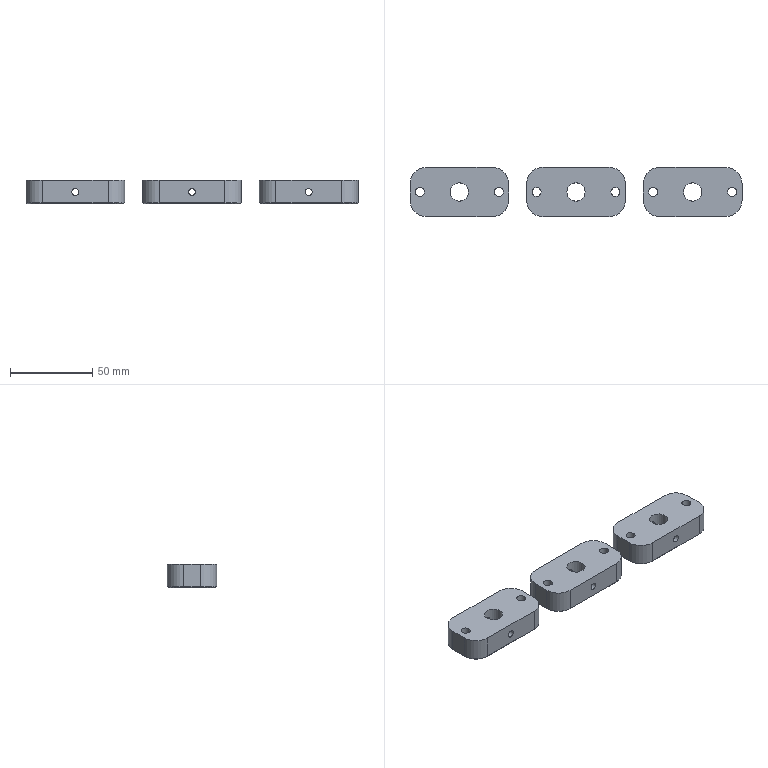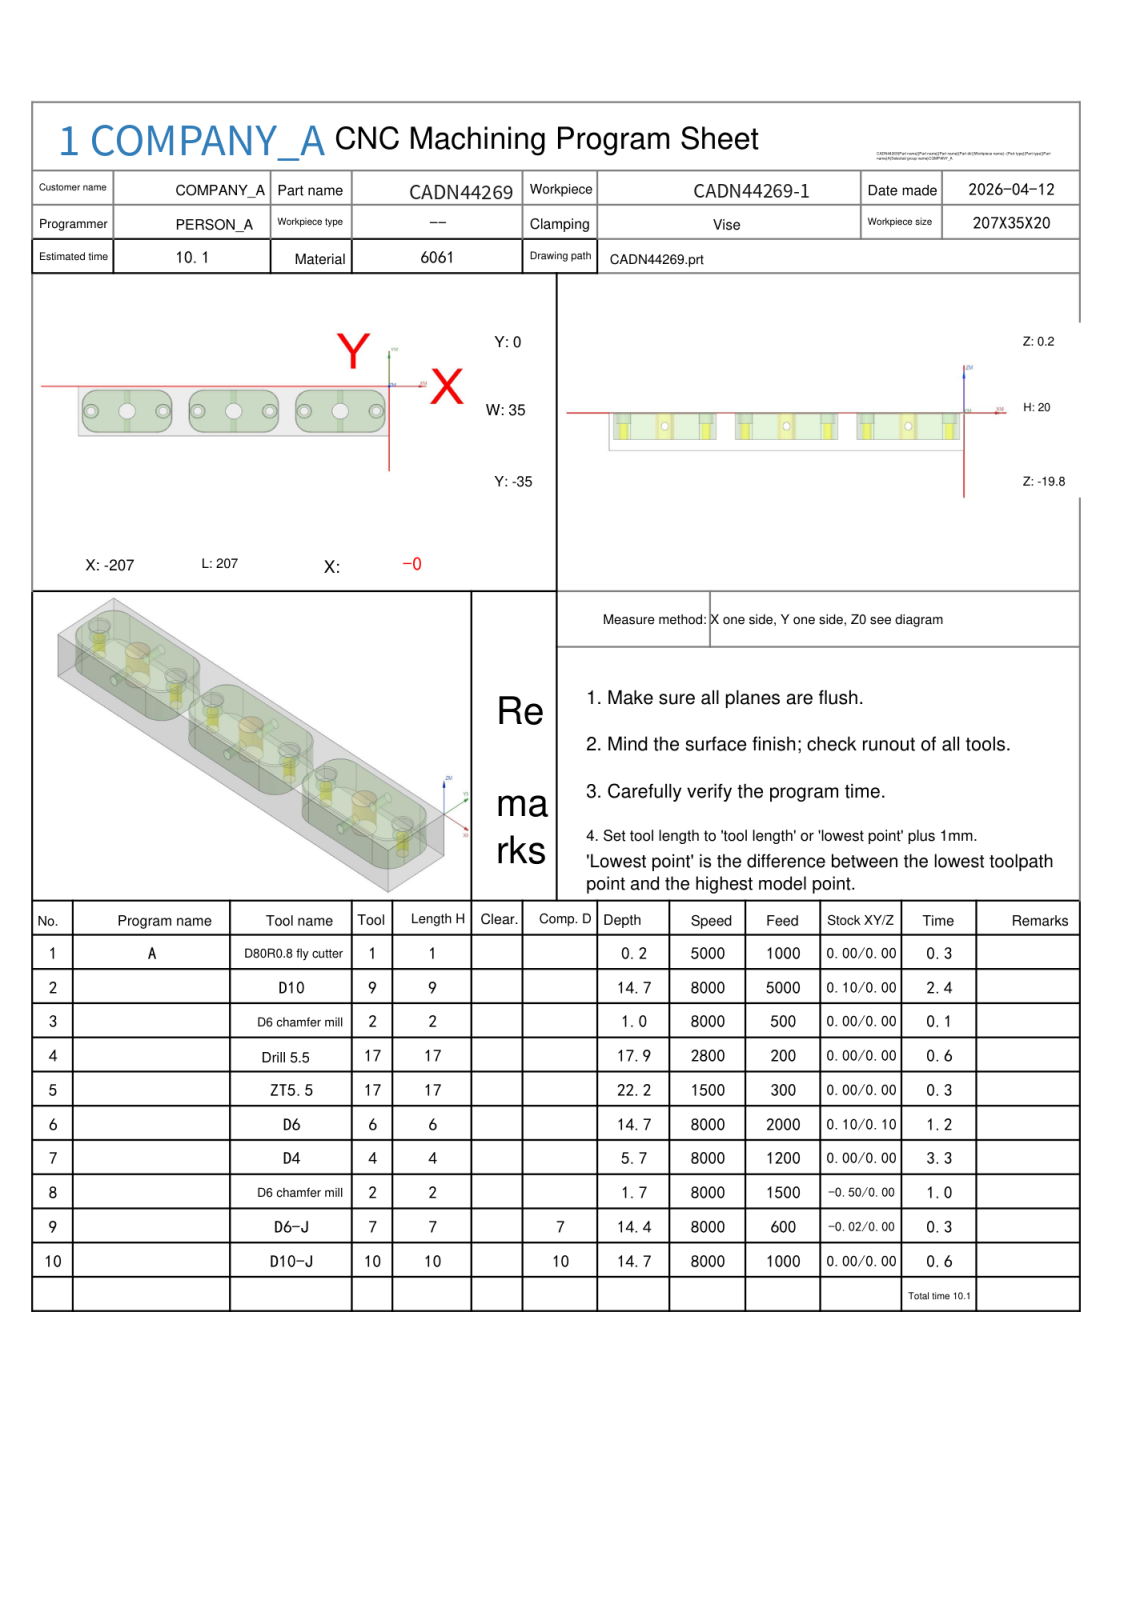NC program | NX | posted by the shop | part box 202 x 30 x 14 mm
Lines 1 to 1289 of 2337, first 1135 of 1287 lines:
%
O0001
(Machine time: 11.90 MIN)
(===Total Tool:8===)
(T1=D80R0.8 fly cutter D=80.  R=0.8  D-  H01 Z=-0.   )
(T9=D10     D=10.  R=0.   D-  H09 Z=-14.5 )
(T2=D6 chamfer mill   D=6.   R=0.   D-  H02 Z=-1.5  )
(T17=drill 5.5  D=5.5  DR_a=118 D-  H17 Z=-22.  )
(T6=D6      D=6.   R=0.   D-  H06 Z=-14.5 )
(T4=D4      D=4.   R=0.   D4  H04 Z=-5.5  )
(T7=D6-J    D=6.   R=0.   D7  H07 Z=-14.2 )
(T10=D10-J  D=10.  R=0.   D10 H10 Z=-14.5 )
G80 G90 G17 G49 G40
G91 G28 Z0
M01
N1 T01 M06
(D80R0.8 fly cutter  D=80. R=0.8 H=01 ce=0.00 di=0.00)
G00 G90 G54 X42.5 Y-17.5 M03 S5000
G43 H01 Z20.
M08
Z2.
G01 Z0.0 F1000.
X37.5
X-244.5
X-249.5
Z2.
G00 Z20.
G91 G28 Z0.0
M05
M09
G91 G28 Z0.0
M01
N2 T09 M06
(D10  D=10. R=0. H=09 ce=0.10 di=0.00)
G00 G90 G54 X-103.5 Y2.6 M03 S8000
G43 H09 Z20.
M08
Z.5
G01 X-83.5 Z.419 F5000.
G02 X-68.4 Y-12.5 Z.323 I0.0 J-15.1
G01 Y-22.5 Z.282
G02 X-83.5 Y-37.6 Z.186 I-15.1 J0.0
G01 X-123.5 Z.024
G02 X-138.6 Y-22.5 Z-.072 I0.0 J15.1
G01 Y-12.5 Z-.112
G02 X-123.5 Y2.6 Z-.208 I15.1 J0.0
G01 X-83.5 Z-.37
G02 X-68.4 Y-12.5 Z-.467 I0.0 J-15.1
G01 Y-22.5 Z-.507
G02 X-83.5 Y-37.6 Z-.603 I-15.1 J0.0
G01 X-123.5 Z-.765
G02 X-138.6 Y-22.5 Z-.861 I0.0 J15.1
G01 Y-12.5 Z-.902
G02 X-123.5 Y2.6 Z-.998 I15.1 J0.0
G01 X-83.5 Z-1.16
G02 X-68.4 Y-12.5 Z-1.256 I0.0 J-15.1
G01 Y-22.5 Z-1.297
G02 X-83.5 Y-37.6 Z-1.393 I-15.1 J0.0
G01 X-123.5 Z-1.555
G02 X-138.6 Y-22.5 Z-1.651 I0.0 J15.1
G01 Y-12.5 Z-1.691
G02 X-123.5 Y2.6 Z-1.787 I15.1 J0.0
G01 X-83.5 Z-1.949
G02 X-68.4 Y-12.5 Z-2.046 I0.0 J-15.1
G01 Y-22.5 Z-2.086
G02 X-83.5 Y-37.6 Z-2.182 I-15.1 J0.0
G01 X-123.5 Z-2.344
G02 X-138.6 Y-22.5 Z-2.44 I0.0 J15.1
G01 Y-12.5 Z-2.481
G02 X-123.5 Y2.6 Z-2.577 I15.1 J0.0
G01 X-83.5 Z-2.739
G02 X-68.4 Y-12.5 Z-2.835 I0.0 J-15.1
G01 Y-22.5 Z-2.876
G02 X-83.5 Y-37.6 Z-2.972 I-15.1 J0.0
G01 X-123.5 Z-3.134
G02 X-138.6 Y-22.5 Z-3.23 I0.0 J15.1
G01 Y-12.5 Z-3.27
G02 X-123.5 Y2.6 Z-3.366 I15.1 J0.0
G01 X-83.5 Z-3.528
G02 X-68.4 Y-12.5 Z-3.624 I0.0 J-15.1
G01 Y-22.5 Z-3.665
G02 X-83.5 Y-37.6 Z-3.761 I-15.1 J0.0
G01 X-123.5 Z-3.923
G02 X-138.6 Y-22.5 Z-4.019 I0.0 J15.1
G01 Y-12.5 Z-4.06
G02 X-123.5 Y2.6 Z-4.156 I15.1 J0.0
G01 X-83.5 Z-4.318
G02 X-68.4 Y-12.5 Z-4.414 I0.0 J-15.1
G01 Y-22.5 Z-4.454
G02 X-83.5 Y-37.6 Z-4.551 I-15.1 J0.0
G01 X-123.5 Z-4.713
G02 X-138.6 Y-22.5 Z-4.809 I0.0 J15.1
G01 Y-12.5 Z-4.849
G02 X-123.5 Y2.6 Z-4.945 I15.1 J0.0
G01 X-83.5 Z-5.107
G02 X-68.4 Y-12.5 Z-5.203 I0.0 J-15.1
G01 Y-22.5 Z-5.244
G02 X-83.5 Y-37.6 Z-5.34 I-15.1 J0.0
G01 X-123.5 Z-5.502
G02 X-138.6 Y-22.5 Z-5.598 I0.0 J15.1
G01 Y-12.5 Z-5.639
G02 X-123.5 Y2.6 Z-5.735 I15.1 J0.0
G01 X-83.5 Z-5.897
G02 X-68.4 Y-12.5 Z-5.993 I0.0 J-15.1
G01 Y-22.5 Z-6.033
G02 X-83.5 Y-37.6 Z-6.13 I-15.1 J0.0
G01 X-123.5 Z-6.292
G02 X-138.6 Y-22.5 Z-6.388 I0.0 J15.1
G01 Y-12.5 Z-6.428
G02 X-123.5 Y2.6 Z-6.524 I15.1 J0.0
G01 X-83.5 Z-6.686
G02 X-68.4 Y-12.5 Z-6.782 I0.0 J-15.1
G01 Y-22.5 Z-6.823
G02 X-83.5 Y-37.6 Z-6.919 I-15.1 J0.0
G01 X-123.5 Z-7.081
G02 X-138.6 Y-22.5 Z-7.177 I0.0 J15.1
G01 Y-12.5 Z-7.218
G02 X-123.5 Y2.6 Z-7.314 I15.1 J0.0
G01 X-83.5 Z-7.476
G02 X-68.4 Y-12.5 Z-7.572 I0.0 J-15.1
G01 Y-22.5 Z-7.612
G02 X-83.5 Y-37.6 Z-7.708 I-15.1 J0.0
G01 X-123.5 Z-7.87
G02 X-138.6 Y-22.5 Z-7.967 I0.0 J15.1
G01 Y-12.5 Z-8.007
G02 X-123.5 Y2.6 Z-8.103 I15.1 J0.0
G01 X-83.5 Z-8.265
G02 X-68.4 Y-12.5 Z-8.361 I0.0 J-15.1
G01 Y-22.5 Z-8.402
G02 X-83.5 Y-37.6 Z-8.498 I-15.1 J0.0
G01 X-123.5 Z-8.66
G02 X-138.6 Y-22.5 Z-8.756 I0.0 J15.1
G01 Y-12.5 Z-8.797
G02 X-123.5 Y2.6 Z-8.893 I15.1 J0.0
G01 X-83.5 Z-9.055
G02 X-68.4 Y-12.5 Z-9.151 I0.0 J-15.1
G01 Y-22.5 Z-9.191
G02 X-83.5 Y-37.6 Z-9.287 I-15.1 J0.0
G01 X-123.5 Z-9.449
G02 X-138.6 Y-22.5 Z-9.546 I0.0 J15.1
G01 Y-12.5 Z-9.586
G02 X-123.5 Y2.6 Z-9.682 I15.1 J0.0
G01 X-83.5 Z-9.844
G02 X-68.4 Y-12.5 Z-9.94 I0.0 J-15.1
G01 Y-22.5 Z-9.981
G02 X-83.5 Y-37.6 Z-10.077 I-15.1 J0.0
G01 X-123.5 Z-10.239
G02 X-138.6 Y-22.5 Z-10.335 I0.0 J15.1
G01 Y-12.5 Z-10.376
G02 X-123.5 Y2.6 Z-10.472 I15.1 J0.0
G01 X-83.5 Z-10.634
G02 X-68.4 Y-12.5 Z-10.73 I0.0 J-15.1
G01 Y-22.5 Z-10.77
G02 X-83.5 Y-37.6 Z-10.866 I-15.1 J0.0
G01 X-123.5 Z-11.028
G02 X-138.6 Y-22.5 Z-11.124 I0.0 J15.1
G01 Y-12.5 Z-11.165
G02 X-123.5 Y2.6 Z-11.261 I15.1 J0.0
G01 X-83.5 Z-11.423
G02 X-68.4 Y-12.5 Z-11.519 I0.0 J-15.1
G01 Y-22.5 Z-11.56
G02 X-83.5 Y-37.6 Z-11.656 I-15.1 J0.0
G01 X-123.5 Z-11.818
G02 X-138.6 Y-22.5 Z-11.914 I0.0 J15.1
G01 Y-12.5 Z-11.954
G02 X-123.5 Y2.6 Z-12.051 I15.1 J0.0
G01 X-83.5 Z-12.213
G02 X-68.4 Y-12.5 Z-12.309 I0.0 J-15.1
G01 Y-22.5 Z-12.349
G02 X-83.5 Y-37.6 Z-12.445 I-15.1 J0.0
G01 X-123.5 Z-12.607
G02 X-138.6 Y-22.5 Z-12.703 I0.0 J15.1
G01 Y-12.5 Z-12.744
G02 X-123.5 Y2.6 Z-12.84 I15.1 J0.0
G01 X-83.5 Z-13.002
G02 X-68.4 Y-12.5 Z-13.098 I0.0 J-15.1
G01 Y-22.5 Z-13.139
G02 X-83.5 Y-37.6 Z-13.235 I-15.1 J0.0
G01 X-123.5 Z-13.397
G02 X-138.6 Y-22.5 Z-13.493 I0.0 J15.1
G01 Y-12.5 Z-13.533
G02 X-123.5 Y2.6 Z-13.63 I15.1 J0.0
G01 X-83.5 Z-13.792
G02 X-68.4 Y-12.5 Z-13.888 I0.0 J-15.1
G01 Y-22.5 Z-13.928
G02 X-83.5 Y-37.6 Z-14.024 I-15.1 J0.0
G01 X-123.5 Z-14.186
G02 X-138.6 Y-22.5 Z-14.282 I0.0 J15.1
G01 Y-12.5 Z-14.323
G02 X-123.5 Y2.6 Z-14.419 I15.1 J0.0
G01 X-103.5 Z-14.5
X-83.5
G02 X-68.4 Y-12.5 I0.0 J-15.1
G01 Y-22.5
G02 X-83.5 Y-37.6 I-15.1 J0.0
G01 X-123.5
G02 X-138.6 Y-22.5 I0.0 J15.1
G01 Y-12.5
G02 X-123.5 Y2.6 I15.1 J0.0
G01 X-103.5
X-103.
Z-13.5
G00 Z20.
X-32.5
Z.5
G01 X-12.5 Z.419
G02 X2.6 Y-12.5 Z.323 I0.0 J-15.1
G01 Y-22.5 Z.282
G02 X-12.5 Y-37.6 Z.186 I-15.1 J0.0
G01 X-52.5 Z.024
G02 X-67.6 Y-22.5 Z-.072 I0.0 J15.1
G01 Y-12.5 Z-.112
G02 X-52.5 Y2.6 Z-.208 I15.1 J0.0
G01 X-12.5 Z-.37
G02 X2.6 Y-12.5 Z-.467 I0.0 J-15.1
G01 Y-22.5 Z-.507
G02 X-12.5 Y-37.6 Z-.603 I-15.1 J0.0
G01 X-52.5 Z-.765
G02 X-67.6 Y-22.5 Z-.861 I0.0 J15.1
G01 Y-12.5 Z-.902
G02 X-52.5 Y2.6 Z-.998 I15.1 J0.0
G01 X-12.5 Z-1.16
G02 X2.6 Y-12.5 Z-1.256 I0.0 J-15.1
G01 Y-22.5 Z-1.297
G02 X-12.5 Y-37.6 Z-1.393 I-15.1 J0.0
G01 X-52.5 Z-1.555
G02 X-67.6 Y-22.5 Z-1.651 I0.0 J15.1
G01 Y-12.5 Z-1.691
G02 X-52.5 Y2.6 Z-1.787 I15.1 J0.0
G01 X-12.5 Z-1.949
G02 X2.6 Y-12.5 Z-2.046 I0.0 J-15.1
G01 Y-22.5 Z-2.086
G02 X-12.5 Y-37.6 Z-2.182 I-15.1 J0.0
G01 X-52.5 Z-2.344
G02 X-67.6 Y-22.5 Z-2.44 I0.0 J15.1
G01 Y-12.5 Z-2.481
G02 X-52.5 Y2.6 Z-2.577 I15.1 J0.0
G01 X-12.5 Z-2.739
G02 X2.6 Y-12.5 Z-2.835 I0.0 J-15.1
G01 Y-22.5 Z-2.876
G02 X-12.5 Y-37.6 Z-2.972 I-15.1 J0.0
G01 X-52.5 Z-3.134
G02 X-67.6 Y-22.5 Z-3.23 I0.0 J15.1
G01 Y-12.5 Z-3.27
G02 X-52.5 Y2.6 Z-3.366 I15.1 J0.0
G01 X-12.5 Z-3.528
G02 X2.6 Y-12.5 Z-3.624 I0.0 J-15.1
G01 Y-22.5 Z-3.665
G02 X-12.5 Y-37.6 Z-3.761 I-15.1 J0.0
G01 X-52.5 Z-3.923
G02 X-67.6 Y-22.5 Z-4.019 I0.0 J15.1
G01 Y-12.5 Z-4.06
G02 X-52.5 Y2.6 Z-4.156 I15.1 J0.0
G01 X-12.5 Z-4.318
G02 X2.6 Y-12.5 Z-4.414 I0.0 J-15.1
G01 Y-22.5 Z-4.454
G02 X-12.5 Y-37.6 Z-4.551 I-15.1 J0.0
G01 X-52.5 Z-4.713
G02 X-67.6 Y-22.5 Z-4.809 I0.0 J15.1
G01 Y-12.5 Z-4.849
G02 X-52.5 Y2.6 Z-4.945 I15.1 J0.0
G01 X-12.5 Z-5.107
G02 X2.6 Y-12.5 Z-5.203 I0.0 J-15.1
G01 Y-22.5 Z-5.244
G02 X-12.5 Y-37.6 Z-5.34 I-15.1 J0.0
G01 X-52.5 Z-5.502
G02 X-67.6 Y-22.5 Z-5.598 I0.0 J15.1
G01 Y-12.5 Z-5.639
G02 X-52.5 Y2.6 Z-5.735 I15.1 J0.0
G01 X-12.5 Z-5.897
G02 X2.6 Y-12.5 Z-5.993 I0.0 J-15.1
G01 Y-22.5 Z-6.033
G02 X-12.5 Y-37.6 Z-6.13 I-15.1 J0.0
G01 X-52.5 Z-6.292
G02 X-67.6 Y-22.5 Z-6.388 I0.0 J15.1
G01 Y-12.5 Z-6.428
G02 X-52.5 Y2.6 Z-6.524 I15.1 J0.0
G01 X-12.5 Z-6.686
G02 X2.6 Y-12.5 Z-6.782 I0.0 J-15.1
G01 Y-22.5 Z-6.823
G02 X-12.5 Y-37.6 Z-6.919 I-15.1 J0.0
G01 X-52.5 Z-7.081
G02 X-67.6 Y-22.5 Z-7.177 I0.0 J15.1
G01 Y-12.5 Z-7.218
G02 X-52.5 Y2.6 Z-7.314 I15.1 J0.0
G01 X-12.5 Z-7.476
G02 X2.6 Y-12.5 Z-7.572 I0.0 J-15.1
G01 Y-22.5 Z-7.612
G02 X-12.5 Y-37.6 Z-7.708 I-15.1 J0.0
G01 X-52.5 Z-7.87
G02 X-67.6 Y-22.5 Z-7.967 I0.0 J15.1
G01 Y-12.5 Z-8.007
G02 X-52.5 Y2.6 Z-8.103 I15.1 J0.0
G01 X-12.5 Z-8.265
G02 X2.6 Y-12.5 Z-8.361 I0.0 J-15.1
G01 Y-22.5 Z-8.402
G02 X-12.5 Y-37.6 Z-8.498 I-15.1 J0.0
G01 X-52.5 Z-8.66
G02 X-67.6 Y-22.5 Z-8.756 I0.0 J15.1
G01 Y-12.5 Z-8.797
G02 X-52.5 Y2.6 Z-8.893 I15.1 J0.0
G01 X-12.5 Z-9.055
G02 X2.6 Y-12.5 Z-9.151 I0.0 J-15.1
G01 Y-22.5 Z-9.191
G02 X-12.5 Y-37.6 Z-9.287 I-15.1 J0.0
G01 X-52.5 Z-9.449
G02 X-67.6 Y-22.5 Z-9.546 I0.0 J15.1
G01 Y-12.5 Z-9.586
G02 X-52.5 Y2.6 Z-9.682 I15.1 J0.0
G01 X-12.5 Z-9.844
G02 X2.6 Y-12.5 Z-9.94 I0.0 J-15.1
G01 Y-22.5 Z-9.981
G02 X-12.5 Y-37.6 Z-10.077 I-15.1 J0.0
G01 X-52.5 Z-10.239
G02 X-67.6 Y-22.5 Z-10.335 I0.0 J15.1
G01 Y-12.5 Z-10.376
G02 X-52.5 Y2.6 Z-10.472 I15.1 J0.0
G01 X-12.5 Z-10.634
G02 X2.6 Y-12.5 Z-10.73 I0.0 J-15.1
G01 Y-22.5 Z-10.77
G02 X-12.5 Y-37.6 Z-10.866 I-15.1 J0.0
G01 X-52.5 Z-11.028
G02 X-67.6 Y-22.5 Z-11.124 I0.0 J15.1
G01 Y-12.5 Z-11.165
G02 X-52.5 Y2.6 Z-11.261 I15.1 J0.0
G01 X-12.5 Z-11.423
G02 X2.6 Y-12.5 Z-11.519 I0.0 J-15.1
G01 Y-22.5 Z-11.56
G02 X-12.5 Y-37.6 Z-11.656 I-15.1 J0.0
G01 X-52.5 Z-11.818
G02 X-67.6 Y-22.5 Z-11.914 I0.0 J15.1
G01 Y-12.5 Z-11.954
G02 X-52.5 Y2.6 Z-12.051 I15.1 J0.0
G01 X-12.5 Z-12.213
G02 X2.6 Y-12.5 Z-12.309 I0.0 J-15.1
G01 Y-22.5 Z-12.349
G02 X-12.5 Y-37.6 Z-12.445 I-15.1 J0.0
G01 X-52.5 Z-12.607
G02 X-67.6 Y-22.5 Z-12.703 I0.0 J15.1
G01 Y-12.5 Z-12.744
G02 X-52.5 Y2.6 Z-12.84 I15.1 J0.0
G01 X-12.5 Z-13.002
G02 X2.6 Y-12.5 Z-13.098 I0.0 J-15.1
G01 Y-22.5 Z-13.139
G02 X-12.5 Y-37.6 Z-13.235 I-15.1 J0.0
G01 X-52.5 Z-13.397
G02 X-67.6 Y-22.5 Z-13.493 I0.0 J15.1
G01 Y-12.5 Z-13.533
G02 X-52.5 Y2.6 Z-13.63 I15.1 J0.0
G01 X-12.5 Z-13.792
G02 X2.6 Y-12.5 Z-13.888 I0.0 J-15.1
G01 Y-22.5 Z-13.928
G02 X-12.5 Y-37.6 Z-14.024 I-15.1 J0.0
G01 X-52.5 Z-14.186
G02 X-67.6 Y-22.5 Z-14.282 I0.0 J15.1
G01 Y-12.5 Z-14.323
G02 X-52.5 Y2.6 Z-14.419 I15.1 J0.0
G01 X-32.5 Z-14.5
X-12.5
G02 X2.6 Y-12.5 I0.0 J-15.1
G01 Y-22.5
G02 X-12.5 Y-37.6 I-15.1 J0.0
G01 X-52.5
G02 X-67.6 Y-22.5 I0.0 J15.1
G01 Y-12.5
G02 X-52.5 Y2.6 I15.1 J0.0
G01 X-32.5
X-32.
Z-13.5
G00 Z20.
X-174.5
Z.5
G01 X-154.5 Z.419
G02 X-139.4 Y-12.5 Z.323 I0.0 J-15.1
G01 Y-22.5 Z.282
G02 X-154.5 Y-37.6 Z.186 I-15.1 J0.0
G01 X-194.5 Z.024
G02 X-209.6 Y-22.5 Z-.072 I0.0 J15.1
G01 Y-12.5 Z-.112
G02 X-194.5 Y2.6 Z-.208 I15.1 J0.0
G01 X-154.5 Z-.37
G02 X-139.4 Y-12.5 Z-.467 I0.0 J-15.1
G01 Y-22.5 Z-.507
G02 X-154.5 Y-37.6 Z-.603 I-15.1 J0.0
G01 X-194.5 Z-.765
G02 X-209.6 Y-22.5 Z-.861 I0.0 J15.1
G01 Y-12.5 Z-.902
G02 X-194.5 Y2.6 Z-.998 I15.1 J0.0
G01 X-154.5 Z-1.16
G02 X-139.4 Y-12.5 Z-1.256 I0.0 J-15.1
G01 Y-22.5 Z-1.297
G02 X-154.5 Y-37.6 Z-1.393 I-15.1 J0.0
G01 X-194.5 Z-1.555
G02 X-209.6 Y-22.5 Z-1.651 I0.0 J15.1
G01 Y-12.5 Z-1.691
G02 X-194.5 Y2.6 Z-1.787 I15.1 J0.0
G01 X-154.5 Z-1.949
G02 X-139.4 Y-12.5 Z-2.046 I0.0 J-15.1
G01 Y-22.5 Z-2.086
G02 X-154.5 Y-37.6 Z-2.182 I-15.1 J0.0
G01 X-194.5 Z-2.344
G02 X-209.6 Y-22.5 Z-2.44 I0.0 J15.1
G01 Y-12.5 Z-2.481
G02 X-194.5 Y2.6 Z-2.577 I15.1 J0.0
G01 X-154.5 Z-2.739
G02 X-139.4 Y-12.5 Z-2.835 I0.0 J-15.1
G01 Y-22.5 Z-2.876
G02 X-154.5 Y-37.6 Z-2.972 I-15.1 J0.0
G01 X-194.5 Z-3.134
G02 X-209.6 Y-22.5 Z-3.23 I0.0 J15.1
G01 Y-12.5 Z-3.27
G02 X-194.5 Y2.6 Z-3.366 I15.1 J0.0
G01 X-154.5 Z-3.528
G02 X-139.4 Y-12.5 Z-3.624 I0.0 J-15.1
G01 Y-22.5 Z-3.665
G02 X-154.5 Y-37.6 Z-3.761 I-15.1 J0.0
G01 X-194.5 Z-3.923
G02 X-209.6 Y-22.5 Z-4.019 I0.0 J15.1
G01 Y-12.5 Z-4.06
G02 X-194.5 Y2.6 Z-4.156 I15.1 J0.0
G01 X-154.5 Z-4.318
G02 X-139.4 Y-12.5 Z-4.414 I0.0 J-15.1
G01 Y-22.5 Z-4.454
G02 X-154.5 Y-37.6 Z-4.551 I-15.1 J0.0
G01 X-194.5 Z-4.713
G02 X-209.6 Y-22.5 Z-4.809 I0.0 J15.1
G01 Y-12.5 Z-4.849
G02 X-194.5 Y2.6 Z-4.945 I15.1 J0.0
G01 X-154.5 Z-5.107
G02 X-139.4 Y-12.5 Z-5.203 I0.0 J-15.1
G01 Y-22.5 Z-5.244
G02 X-154.5 Y-37.6 Z-5.34 I-15.1 J0.0
G01 X-194.5 Z-5.502
G02 X-209.6 Y-22.5 Z-5.598 I0.0 J15.1
G01 Y-12.5 Z-5.639
G02 X-194.5 Y2.6 Z-5.735 I15.1 J0.0
G01 X-154.5 Z-5.897
G02 X-139.4 Y-12.5 Z-5.993 I0.0 J-15.1
G01 Y-22.5 Z-6.033
G02 X-154.5 Y-37.6 Z-6.13 I-15.1 J0.0
G01 X-194.5 Z-6.292
G02 X-209.6 Y-22.5 Z-6.388 I0.0 J15.1
G01 Y-12.5 Z-6.428
G02 X-194.5 Y2.6 Z-6.524 I15.1 J0.0
G01 X-154.5 Z-6.686
G02 X-139.4 Y-12.5 Z-6.782 I0.0 J-15.1
G01 Y-22.5 Z-6.823
G02 X-154.5 Y-37.6 Z-6.919 I-15.1 J0.0
G01 X-194.5 Z-7.081
G02 X-209.6 Y-22.5 Z-7.177 I0.0 J15.1
G01 Y-12.5 Z-7.218
G02 X-194.5 Y2.6 Z-7.314 I15.1 J0.0
G01 X-154.5 Z-7.476
G02 X-139.4 Y-12.5 Z-7.572 I0.0 J-15.1
G01 Y-22.5 Z-7.612
G02 X-154.5 Y-37.6 Z-7.708 I-15.1 J0.0
G01 X-194.5 Z-7.87
G02 X-209.6 Y-22.5 Z-7.967 I0.0 J15.1
G01 Y-12.5 Z-8.007
G02 X-194.5 Y2.6 Z-8.103 I15.1 J0.0
G01 X-154.5 Z-8.265
G02 X-139.4 Y-12.5 Z-8.361 I0.0 J-15.1
G01 Y-22.5 Z-8.402
G02 X-154.5 Y-37.6 Z-8.498 I-15.1 J0.0
G01 X-194.5 Z-8.66
G02 X-209.6 Y-22.5 Z-8.756 I0.0 J15.1
G01 Y-12.5 Z-8.797
G02 X-194.5 Y2.6 Z-8.893 I15.1 J0.0
G01 X-154.5 Z-9.055
G02 X-139.4 Y-12.5 Z-9.151 I0.0 J-15.1
G01 Y-22.5 Z-9.191
G02 X-154.5 Y-37.6 Z-9.287 I-15.1 J0.0
G01 X-194.5 Z-9.449
G02 X-209.6 Y-22.5 Z-9.546 I0.0 J15.1
G01 Y-12.5 Z-9.586
G02 X-194.5 Y2.6 Z-9.682 I15.1 J0.0
G01 X-154.5 Z-9.844
G02 X-139.4 Y-12.5 Z-9.94 I0.0 J-15.1
G01 Y-22.5 Z-9.981
G02 X-154.5 Y-37.6 Z-10.077 I-15.1 J0.0
G01 X-194.5 Z-10.239
G02 X-209.6 Y-22.5 Z-10.335 I0.0 J15.1
G01 Y-12.5 Z-10.376
G02 X-194.5 Y2.6 Z-10.472 I15.1 J0.0
G01 X-154.5 Z-10.634
G02 X-139.4 Y-12.5 Z-10.73 I0.0 J-15.1
G01 Y-22.5 Z-10.77
G02 X-154.5 Y-37.6 Z-10.866 I-15.1 J0.0
G01 X-194.5 Z-11.028
G02 X-209.6 Y-22.5 Z-11.124 I0.0 J15.1
G01 Y-12.5 Z-11.165
G02 X-194.5 Y2.6 Z-11.261 I15.1 J0.0
G01 X-154.5 Z-11.423
G02 X-139.4 Y-12.5 Z-11.519 I0.0 J-15.1
G01 Y-22.5 Z-11.56
G02 X-154.5 Y-37.6 Z-11.656 I-15.1 J0.0
G01 X-194.5 Z-11.818
G02 X-209.6 Y-22.5 Z-11.914 I0.0 J15.1
G01 Y-12.5 Z-11.954
G02 X-194.5 Y2.6 Z-12.051 I15.1 J0.0
G01 X-154.5 Z-12.213
G02 X-139.4 Y-12.5 Z-12.309 I0.0 J-15.1
G01 Y-22.5 Z-12.349
G02 X-154.5 Y-37.6 Z-12.445 I-15.1 J0.0
G01 X-194.5 Z-12.607
G02 X-209.6 Y-22.5 Z-12.703 I0.0 J15.1
G01 Y-12.5 Z-12.744
G02 X-194.5 Y2.6 Z-12.84 I15.1 J0.0
G01 X-154.5 Z-13.002
G02 X-139.4 Y-12.5 Z-13.098 I0.0 J-15.1
G01 Y-22.5 Z-13.139
G02 X-154.5 Y-37.6 Z-13.235 I-15.1 J0.0
G01 X-194.5 Z-13.397
G02 X-209.6 Y-22.5 Z-13.493 I0.0 J15.1
G01 Y-12.5 Z-13.533
G02 X-194.5 Y2.6 Z-13.63 I15.1 J0.0
G01 X-154.5 Z-13.792
G02 X-139.4 Y-12.5 Z-13.888 I0.0 J-15.1
G01 Y-22.5 Z-13.928
G02 X-154.5 Y-37.6 Z-14.024 I-15.1 J0.0
G01 X-194.5 Z-14.186
G02 X-209.6 Y-22.5 Z-14.282 I0.0 J15.1
G01 Y-12.5 Z-14.323
G02 X-194.5 Y2.6 Z-14.419 I15.1 J0.0
G01 X-174.5 Z-14.5
X-154.5
G02 X-139.4 Y-12.5 I0.0 J-15.1
G01 Y-22.5
G02 X-154.5 Y-37.6 I-15.1 J0.0
G01 X-194.5
G02 X-209.6 Y-22.5 I0.0 J15.1
G01 Y-12.5
G02 X-194.5 Y2.6 I15.1 J0.0
G01 X-174.5
X-174.
Z-13.5
G00 Z20.
G91 G28 Z0.0
M05
M09
G91 G28 Z0.0
M01
N3 T02 M06
(D6 chamfer mill  D=6. R=0. H=02 ce=0.00 di=0.00)
G00 G90 G54 X-174.5 Y-17.5 M03 S8000
G43 H02 Z20.
M08
G98 G82 X-174.5 Y-17.5 Z-.8 R1. F500.
X-103.5
X-32.5
G80
G00 Z20.
G00 G90 X-198.5 Y-17.5 M03 S8000
Z20.
G98 G81 X-198.5 Y-17.5 Z-.8 R1. F500.
X-150.5
X-127.5
X-79.5
X-56.5
X-8.5
G80
G00 Z20.
G91 G28 Z0.0
M05
M09
G91 G28 Z0.0
M01
N4 T17 M06
(drill 5.5 D=5.5 DR_a=118 H=17)
G00 G90 G54 X-198.5 Y-17.5 M03 S2800
G43 H17 Z20.
M08
G98 G83 X-198.5 Y-17.5 Z-17.652 R1. F200. Q2.
X-150.5
X-127.5
X-79.5
X-56.5
X-8.5
G80
G00 Z20.
G91 G28 Z0.0
M05
M09
G91 G28 Z0.0
M01
N5 T17 M06
(ZT5.5 D=5.5 DR_a=118 H=17)
G00 G90 G54 X-174.5 Y-17.5 M03 S1500
G43 H17 Z20.
M08
G98 G83 X-174.5 Y-17.5 Z-22. R1. F300. Q3.
X-103.5
X-32.5
G80
G00 Z20.
G91 G28 Z0.0
M05
M09
G91 G28 Z0.0
M01
N6 T06 M06
(D6  D=6. R=0. H=06 ce=0.10 di=0.10)
G00 G90 G54 X-34.93 Y-17.611 M03 S8000
G43 H06 Z20.
M08
Z1.
G01 Y-17.883 Z.986 F2000.
X-34.563 Y-18.839 Z.932
X-33.839 Y-19.563 Z.878
X-32.883 Y-19.93 Z.825
X-32.117 Z.785
X-31.161 Y-19.563 Z.731
X-30.437 Y-18.839 Z.677
X-30.07 Y-17.883 Z.624
Y-17.117 Z.583
X-30.437 Y-16.161 Z.53
X-31.161 Y-15.437 Z.476
X-32.117 Y-15.07 Z.422
X-32.883 Z.382
X-33.839 Y-15.437 Z.329
X-34.563 Y-16.161 Z.275
X-34.93 Y-17.117 Z.221
Y-17.883 Z.181
X-34.563 Y-18.839 Z.127
X-33.839 Y-19.563 Z.074
X-32.883 Y-19.93 Z.02
X-32.5 Z0.0
G03 X-30.07 Y-17.5 Z-.074 I0.0 J2.43
X-32.5 Y-15.07 Z-.148 I-2.43 J0.0
X-34.93 Y-17.5 Z-.222 I0.0 J-2.43
X-32.5 Y-19.93 Z-.296 I2.43 J0.0
X-30.07 Y-17.5 Z-.37 I0.0 J2.43
X-32.5 Y-15.07 Z-.444 I-2.43 J0.0
X-34.93 Y-17.5 Z-.518 I0.0 J-2.43
X-32.5 Y-19.93 Z-.592 I2.43 J0.0
X-30.07 Y-17.5 Z-.666 I0.0 J2.43
X-32.5 Y-15.07 Z-.74 I-2.43 J0.0
X-34.93 Y-17.5 Z-.814 I0.0 J-2.43
X-32.5 Y-19.93 Z-.888 I2.43 J0.0
X-30.07 Y-17.5 Z-.962 I0.0 J2.43
X-32.5 Y-15.07 Z-1.036 I-2.43 J0.0
X-34.93 Y-17.5 Z-1.11 I0.0 J-2.43
X-32.5 Y-19.93 Z-1.184 I2.43 J0.0
X-30.07 Y-17.5 Z-1.258 I0.0 J2.43
X-32.5 Y-15.07 Z-1.332 I-2.43 J0.0
X-34.93 Y-17.5 Z-1.406 I0.0 J-2.43
X-32.5 Y-19.93 Z-1.48 I2.43 J0.0
X-30.07 Y-17.5 Z-1.554 I0.0 J2.43
X-32.5 Y-15.07 Z-1.628 I-2.43 J0.0
X-34.93 Y-17.5 Z-1.702 I0.0 J-2.43
X-32.5 Y-19.93 Z-1.776 I2.43 J0.0
X-30.07 Y-17.5 Z-1.849 I0.0 J2.43
X-32.5 Y-15.07 Z-1.923 I-2.43 J0.0
X-34.93 Y-17.5 Z-1.997 I0.0 J-2.43
X-32.5 Y-19.93 Z-2.071 I2.43 J0.0
X-30.07 Y-17.5 Z-2.145 I0.0 J2.43
X-32.5 Y-15.07 Z-2.219 I-2.43 J0.0
X-34.93 Y-17.5 Z-2.293 I0.0 J-2.43
X-32.5 Y-19.93 Z-2.367 I2.43 J0.0
X-30.07 Y-17.5 Z-2.441 I0.0 J2.43
X-32.5 Y-15.07 Z-2.515 I-2.43 J0.0
X-34.93 Y-17.5 Z-2.589 I0.0 J-2.43
X-32.5 Y-19.93 Z-2.663 I2.43 J0.0
X-30.07 Y-17.5 Z-2.737 I0.0 J2.43
X-32.5 Y-15.07 Z-2.811 I-2.43 J0.0
X-34.93 Y-17.5 Z-2.885 I0.0 J-2.43
X-32.5 Y-19.93 Z-2.959 I2.43 J0.0
X-30.07 Y-17.5 Z-3.033 I0.0 J2.43
X-32.5 Y-15.07 Z-3.107 I-2.43 J0.0
X-34.93 Y-17.5 Z-3.181 I0.0 J-2.43
X-32.5 Y-19.93 Z-3.255 I2.43 J0.0
X-30.07 Y-17.5 Z-3.329 I0.0 J2.43
X-32.5 Y-15.07 Z-3.403 I-2.43 J0.0
X-34.93 Y-17.5 Z-3.477 I0.0 J-2.43
X-32.5 Y-19.93 Z-3.551 I2.43 J0.0
X-30.07 Y-17.5 Z-3.625 I0.0 J2.43
X-32.5 Y-15.07 Z-3.699 I-2.43 J0.0
X-34.93 Y-17.5 Z-3.773 I0.0 J-2.43
X-32.5 Y-19.93 Z-3.847 I2.43 J0.0
X-30.07 Y-17.5 Z-3.921 I0.0 J2.43
X-32.5 Y-15.07 Z-3.995 I-2.43 J0.0
X-34.93 Y-17.5 Z-4.069 I0.0 J-2.43
X-32.5 Y-19.93 Z-4.143 I2.43 J0.0
X-30.07 Y-17.5 Z-4.217 I0.0 J2.43
X-32.5 Y-15.07 Z-4.291 I-2.43 J0.0
X-34.93 Y-17.5 Z-4.365 I0.0 J-2.43
X-32.5 Y-19.93 Z-4.439 I2.43 J0.0
X-30.07 Y-17.5 Z-4.513 I0.0 J2.43
X-32.5 Y-15.07 Z-4.587 I-2.43 J0.0
X-34.93 Y-17.5 Z-4.661 I0.0 J-2.43
X-32.5 Y-19.93 Z-4.735 I2.43 J0.0
X-30.07 Y-17.5 Z-4.809 I0.0 J2.43
X-32.5 Y-15.07 Z-4.883 I-2.43 J0.0
X-34.93 Y-17.5 Z-4.957 I0.0 J-2.43
X-32.5 Y-19.93 Z-5.031 I2.43 J0.0
X-30.07 Y-17.5 Z-5.105 I0.0 J2.43
X-32.5 Y-15.07 Z-5.179 I-2.43 J0.0
X-34.93 Y-17.5 Z-5.253 I0.0 J-2.43
X-32.5 Y-19.93 Z-5.327 I2.43 J0.0
X-30.07 Y-17.5 Z-5.401 I0.0 J2.43
X-32.5 Y-15.07 Z-5.474 I-2.43 J0.0
X-34.93 Y-17.5 Z-5.548 I0.0 J-2.43
X-32.5 Y-19.93 Z-5.622 I2.43 J0.0
X-30.07 Y-17.5 Z-5.696 I0.0 J2.43
X-32.5 Y-15.07 Z-5.77 I-2.43 J0.0
X-34.93 Y-17.5 Z-5.844 I0.0 J-2.43
X-32.5 Y-19.93 Z-5.918 I2.43 J0.0
X-30.07 Y-17.5 Z-5.992 I0.0 J2.43
X-32.5 Y-15.07 Z-6.066 I-2.43 J0.0
X-34.93 Y-17.5 Z-6.14 I0.0 J-2.43
X-32.5 Y-19.93 Z-6.214 I2.43 J0.0
X-30.07 Y-17.5 Z-6.288 I0.0 J2.43
X-32.5 Y-15.07 Z-6.362 I-2.43 J0.0
X-34.93 Y-17.5 Z-6.436 I0.0 J-2.43
X-32.5 Y-19.93 Z-6.51 I2.43 J0.0
X-30.07 Y-17.5 Z-6.584 I0.0 J2.43
X-32.5 Y-15.07 Z-6.658 I-2.43 J0.0
X-34.93 Y-17.5 Z-6.732 I0.0 J-2.43
X-32.5 Y-19.93 Z-6.806 I2.43 J0.0
X-30.07 Y-17.5 Z-6.88 I0.0 J2.43
X-32.5 Y-15.07 Z-6.954 I-2.43 J0.0
X-34.93 Y-17.5 Z-7.028 I0.0 J-2.43
X-32.5 Y-19.93 Z-7.102 I2.43 J0.0
X-30.07 Y-17.5 Z-7.176 I0.0 J2.43
X-32.5 Y-15.07 Z-7.25 I-2.43 J0.0
X-34.93 Y-17.5 Z-7.324 I0.0 J-2.43
X-32.5 Y-19.93 Z-7.398 I2.43 J0.0
X-30.07 Y-17.5 Z-7.472 I0.0 J2.43
X-32.5 Y-15.07 Z-7.546 I-2.43 J0.0
X-34.93 Y-17.5 Z-7.62 I0.0 J-2.43
X-32.5 Y-19.93 Z-7.694 I2.43 J0.0
X-30.07 Y-17.5 Z-7.768 I0.0 J2.43
X-32.5 Y-15.07 Z-7.842 I-2.43 J0.0
X-34.93 Y-17.5 Z-7.916 I0.0 J-2.43
X-32.5 Y-19.93 Z-7.99 I2.43 J0.0
X-30.07 Y-17.5 Z-8.064 I0.0 J2.43
X-32.5 Y-15.07 Z-8.138 I-2.43 J0.0
X-34.93 Y-17.5 Z-8.212 I0.0 J-2.43
X-32.5 Y-19.93 Z-8.286 I2.43 J0.0
X-30.07 Y-17.5 Z-8.36 I0.0 J2.43
X-32.5 Y-15.07 Z-8.434 I-2.43 J0.0
X-34.93 Y-17.5 Z-8.508 I0.0 J-2.43
X-32.5 Y-19.93 Z-8.582 I2.43 J0.0
X-30.07 Y-17.5 Z-8.656 I0.0 J2.43
X-32.5 Y-15.07 Z-8.73 I-2.43 J0.0
X-34.93 Y-17.5 Z-8.804 I0.0 J-2.43
X-32.5 Y-19.93 Z-8.878 I2.43 J0.0
X-30.07 Y-17.5 Z-8.952 I0.0 J2.43
X-32.5 Y-15.07 Z-9.026 I-2.43 J0.0
X-34.93 Y-17.5 Z-9.099 I0.0 J-2.43
X-32.5 Y-19.93 Z-9.173 I2.43 J0.0
X-30.07 Y-17.5 Z-9.247 I0.0 J2.43
X-32.5 Y-15.07 Z-9.321 I-2.43 J0.0
X-34.93 Y-17.5 Z-9.395 I0.0 J-2.43
X-32.5 Y-19.93 Z-9.469 I2.43 J0.0
X-30.07 Y-17.5 Z-9.543 I0.0 J2.43
X-32.5 Y-15.07 Z-9.617 I-2.43 J0.0
X-34.93 Y-17.5 Z-9.691 I0.0 J-2.43
X-32.5 Y-19.93 Z-9.765 I2.43 J0.0
X-30.07 Y-17.5 Z-9.839 I0.0 J2.43
X-32.5 Y-15.07 Z-9.913 I-2.43 J0.0
X-34.93 Y-17.5 Z-9.987 I0.0 J-2.43
X-32.5 Y-19.93 Z-10.061 I2.43 J0.0
X-30.07 Y-17.5 Z-10.135 I0.0 J2.43
X-32.5 Y-15.07 Z-10.209 I-2.43 J0.0
X-34.93 Y-17.5 Z-10.283 I0.0 J-2.43
X-32.5 Y-19.93 Z-10.357 I2.43 J0.0
X-30.07 Y-17.5 Z-10.431 I0.0 J2.43
X-32.5 Y-15.07 Z-10.505 I-2.43 J0.0
X-34.93 Y-17.5 Z-10.579 I0.0 J-2.43
X-32.5 Y-19.93 Z-10.653 I2.43 J0.0
X-30.07 Y-17.5 Z-10.727 I0.0 J2.43
X-32.5 Y-15.07 Z-10.801 I-2.43 J0.0
X-34.93 Y-17.5 Z-10.875 I0.0 J-2.43
X-32.5 Y-19.93 Z-10.949 I2.43 J0.0
X-30.07 Y-17.5 Z-11.023 I0.0 J2.43
X-32.5 Y-15.07 Z-11.097 I-2.43 J0.0
X-34.93 Y-17.5 Z-11.171 I0.0 J-2.43
X-32.5 Y-19.93 Z-11.245 I2.43 J0.0
X-30.07 Y-17.5 Z-11.319 I0.0 J2.43
X-32.5 Y-15.07 Z-11.393 I-2.43 J0.0
X-34.93 Y-17.5 Z-11.467 I0.0 J-2.43
X-32.5 Y-19.93 Z-11.541 I2.43 J0.0
X-30.07 Y-17.5 Z-11.615 I0.0 J2.43
X-32.5 Y-15.07 Z-11.689 I-2.43 J0.0
X-34.93 Y-17.5 Z-11.763 I0.0 J-2.43
X-32.5 Y-19.93 Z-11.837 I2.43 J0.0
X-30.07 Y-17.5 Z-11.911 I0.0 J2.43
X-32.5 Y-15.07 Z-11.985 I-2.43 J0.0
X-34.93 Y-17.5 Z-12.059 I0.0 J-2.43
X-32.5 Y-19.93 Z-12.133 I2.43 J0.0
X-30.07 Y-17.5 Z-12.207 I0.0 J2.43
X-32.5 Y-15.07 Z-12.281 I-2.43 J0.0
X-34.93 Y-17.5 Z-12.355 I0.0 J-2.43
X-32.5 Y-19.93 Z-12.429 I2.43 J0.0
X-30.07 Y-17.5 Z-12.503 I0.0 J2.43
X-32.5 Y-15.07 Z-12.577 I-2.43 J0.0
X-34.93 Y-17.5 Z-12.651 I0.0 J-2.43
X-32.5 Y-19.93 Z-12.724 I2.43 J0.0
X-30.07 Y-17.5 Z-12.798 I0.0 J2.43
X-32.5 Y-15.07 Z-12.872 I-2.43 J0.0
X-34.93 Y-17.5 Z-12.946 I0.0 J-2.43
X-32.5 Y-19.93 Z-13.02 I2.43 J0.0
X-30.07 Y-17.5 Z-13.094 I0.0 J2.43
X-32.5 Y-15.07 Z-13.168 I-2.43 J0.0
X-34.93 Y-17.5 Z-13.242 I0.0 J-2.43
X-32.5 Y-19.93 Z-13.316 I2.43 J0.0
X-30.07 Y-17.5 Z-13.39 I0.0 J2.43
X-32.5 Y-15.07 Z-13.464 I-2.43 J0.0
X-34.93 Y-17.5 Z-13.538 I0.0 J-2.43
X-32.5 Y-19.93 Z-13.612 I2.43 J0.0
X-30.07 Y-17.5 Z-13.686 I0.0 J2.43
X-32.5 Y-15.07 Z-13.76 I-2.43 J0.0
X-34.93 Y-17.5 Z-13.834 I0.0 J-2.43
X-32.5 Y-19.93 Z-13.908 I2.43 J0.0
X-30.07 Y-17.5 Z-13.982 I0.0 J2.43
X-32.5 Y-15.07 Z-14.056 I-2.43 J0.0
X-34.93 Y-17.5 Z-14.13 I0.0 J-2.43
X-32.5 Y-19.93 Z-14.204 I2.43 J0.0
X-30.07 Y-17.5 Z-14.278 I0.0 J2.43
X-32.5 Y-15.07 Z-14.352 I-2.43 J0.0
X-34.93 Y-17.5 Z-14.426 I0.0 J-2.43
X-32.5 Y-19.93 Z-14.5 I2.43 J0.0
X-30.07 Y-17.5 I0.0 J2.43
X-32.5 Y-15.07 I-2.43 J0.0
X-34.93 Y-17.5 I0.0 J-2.43
X-32.5 Y-19.93 I2.43 J0.0
X-32.102 Y-19.897 I0.0 J2.43
G01 Z-13.5
G00 Z20.
X-105.93 Y-17.611
Z1.
G01 Y-17.883 Z.986
X-105.563 Y-18.839 Z.932
X-104.839 Y-19.563 Z.878
X-103.883 Y-19.93 Z.825
X-103.117 Z.785
X-102.161 Y-19.563 Z.731
X-101.437 Y-18.839 Z.677
X-101.07 Y-17.883 Z.624
Y-17.117 Z.583
X-101.437 Y-16.161 Z.53
X-102.161 Y-15.437 Z.476
X-103.117 Y-15.07 Z.422
X-103.883 Z.382
X-104.839 Y-15.437 Z.329
X-105.563 Y-16.161 Z.275
X-105.93 Y-17.117 Z.221
Y-17.883 Z.181
X-105.563 Y-18.839 Z.127
X-104.839 Y-19.563 Z.074
X-103.883 Y-19.93 Z.02
X-103.5 Z0.0
G03 X-101.07 Y-17.5 Z-.074 I0.0 J2.43
X-103.5 Y-15.07 Z-.148 I-2.43 J0.0
X-105.93 Y-17.5 Z-.222 I0.0 J-2.43
X-103.5 Y-19.93 Z-.296 I2.43 J0.0
X-101.07 Y-17.5 Z-.37 I0.0 J2.43
X-103.5 Y-15.07 Z-.444 I-2.43 J0.0
X-105.93 Y-17.5 Z-.518 I0.0 J-2.43
X-103.5 Y-19.93 Z-.592 I2.43 J0.0
X-101.07 Y-17.5 Z-.666 I0.0 J2.43
X-103.5 Y-15.07 Z-.74 I-2.43 J0.0
X-105.93 Y-17.5 Z-.814 I0.0 J-2.43
X-103.5 Y-19.93 Z-.888 I2.43 J0.0
X-101.07 Y-17.5 Z-.962 I0.0 J2.43
X-103.5 Y-15.07 Z-1.036 I-2.43 J0.0
X-105.93 Y-17.5 Z-1.11 I0.0 J-2.43
X-103.5 Y-19.93 Z-1.184 I2.43 J0.0
X-101.07 Y-17.5 Z-1.258 I0.0 J2.43
X-103.5 Y-15.07 Z-1.332 I-2.43 J0.0
X-105.93 Y-17.5 Z-1.406 I0.0 J-2.43
X-103.5 Y-19.93 Z-1.48 I2.43 J0.0
X-101.07 Y-17.5 Z-1.554 I0.0 J2.43
X-103.5 Y-15.07 Z-1.628 I-2.43 J0.0
X-105.93 Y-17.5 Z-1.702 I0.0 J-2.43
X-103.5 Y-19.93 Z-1.776 I2.43 J0.0
X-101.07 Y-17.5 Z-1.849 I0.0 J2.43
X-103.5 Y-15.07 Z-1.923 I-2.43 J0.0
X-105.93 Y-17.5 Z-1.997 I0.0 J-2.43
X-103.5 Y-19.93 Z-2.071 I2.43 J0.0
X-101.07 Y-17.5 Z-2.145 I0.0 J2.43
X-103.5 Y-15.07 Z-2.219 I-2.43 J0.0
X-105.93 Y-17.5 Z-2.293 I0.0 J-2.43
X-103.5 Y-19.93 Z-2.367 I2.43 J0.0
X-101.07 Y-17.5 Z-2.441 I0.0 J2.43
X-103.5 Y-15.07 Z-2.515 I-2.43 J0.0
X-105.93 Y-17.5 Z-2.589 I0.0 J-2.43
X-103.5 Y-19.93 Z-2.663 I2.43 J0.0
X-101.07 Y-17.5 Z-2.737 I0.0 J2.43
X-103.5 Y-15.07 Z-2.811 I-2.43 J0.0
X-105.93 Y-17.5 Z-2.885 I0.0 J-2.43
X-103.5 Y-19.93 Z-2.959 I2.43 J0.0
X-101.07 Y-17.5 Z-3.033 I0.0 J2.43
X-103.5 Y-15.07 Z-3.107 I-2.43 J0.0
X-105.93 Y-17.5 Z-3.181 I0.0 J-2.43
X-103.5 Y-19.93 Z-3.255 I2.43 J0.0
X-101.07 Y-17.5 Z-3.329 I0.0 J2.43
X-103.5 Y-15.07 Z-3.403 I-2.43 J0.0
X-105.93 Y-17.5 Z-3.477 I0.0 J-2.43
X-103.5 Y-19.93 Z-3.551 I2.43 J0.0
X-101.07 Y-17.5 Z-3.625 I0.0 J2.43
X-103.5 Y-15.07 Z-3.699 I-2.43 J0.0
X-105.93 Y-17.5 Z-3.773 I0.0 J-2.43
X-103.5 Y-19.93 Z-3.847 I2.43 J0.0
X-101.07 Y-17.5 Z-3.921 I0.0 J2.43
X-103.5 Y-15.07 Z-3.995 I-2.43 J0.0
X-105.93 Y-17.5 Z-4.069 I0.0 J-2.43
X-103.5 Y-19.93 Z-4.143 I2.43 J0.0
X-101.07 Y-17.5 Z-4.217 I0.0 J2.43
X-103.5 Y-15.07 Z-4.291 I-2.43 J0.0
X-105.93 Y-17.5 Z-4.365 I0.0 J-2.43
X-103.5 Y-19.93 Z-4.439 I2.43 J0.0
X-101.07 Y-17.5 Z-4.513 I0.0 J2.43
X-103.5 Y-15.07 Z-4.587 I-2.43 J0.0
X-105.93 Y-17.5 Z-4.661 I0.0 J-2.43
X-103.5 Y-19.93 Z-4.735 I2.43 J0.0
X-101.07 Y-17.5 Z-4.809 I0.0 J2.43
X-103.5 Y-15.07 Z-4.883 I-2.43 J0.0
X-105.93 Y-17.5 Z-4.957 I0.0 J-2.43
X-103.5 Y-19.93 Z-5.031 I2.43 J0.0
X-101.07 Y-17.5 Z-5.105 I0.0 J2.43
X-103.5 Y-15.07 Z-5.179 I-2.43 J0.0
X-105.93 Y-17.5 Z-5.253 I0.0 J-2.43
X-103.5 Y-19.93 Z-5.327 I2.43 J0.0
X-101.07 Y-17.5 Z-5.401 I0.0 J2.43
X-103.5 Y-15.07 Z-5.474 I-2.43 J0.0
X-105.93 Y-17.5 Z-5.548 I0.0 J-2.43
X-103.5 Y-19.93 Z-5.622 I2.43 J0.0
X-101.07 Y-17.5 Z-5.696 I0.0 J2.43
X-103.5 Y-15.07 Z-5.77 I-2.43 J0.0
X-105.93 Y-17.5 Z-5.844 I0.0 J-2.43
X-103.5 Y-19.93 Z-5.918 I2.43 J0.0
X-101.07 Y-17.5 Z-5.992 I0.0 J2.43
X-103.5 Y-15.07 Z-6.066 I-2.43 J0.0
X-105.93 Y-17.5 Z-6.14 I0.0 J-2.43
X-103.5 Y-19.93 Z-6.214 I2.43 J0.0
X-101.07 Y-17.5 Z-6.288 I0.0 J2.43
X-103.5 Y-15.07 Z-6.362 I-2.43 J0.0
X-105.93 Y-17.5 Z-6.436 I0.0 J-2.43
X-103.5 Y-19.93 Z-6.51 I2.43 J0.0
X-101.07 Y-17.5 Z-6.584 I0.0 J2.43
X-103.5 Y-15.07 Z-6.658 I-2.43 J0.0
X-105.93 Y-17.5 Z-6.732 I0.0 J-2.43
X-103.5 Y-19.93 Z-6.806 I2.43 J0.0
X-101.07 Y-17.5 Z-6.88 I0.0 J2.43
X-103.5 Y-15.07 Z-6.954 I-2.43 J0.0
X-105.93 Y-17.5 Z-7.028 I0.0 J-2.43
X-103.5 Y-19.93 Z-7.102 I2.43 J0.0
X-101.07 Y-17.5 Z-7.176 I0.0 J2.43
X-103.5 Y-15.07 Z-7.25 I-2.43 J0.0
X-105.93 Y-17.5 Z-7.324 I0.0 J-2.43
X-103.5 Y-19.93 Z-7.398 I2.43 J0.0
X-101.07 Y-17.5 Z-7.472 I0.0 J2.43
X-103.5 Y-15.07 Z-7.546 I-2.43 J0.0
X-105.93 Y-17.5 Z-7.62 I0.0 J-2.43
X-103.5 Y-19.93 Z-7.694 I2.43 J0.0
X-101.07 Y-17.5 Z-7.768 I0.0 J2.43
X-103.5 Y-15.07 Z-7.842 I-2.43 J0.0
X-105.93 Y-17.5 Z-7.916 I0.0 J-2.43
X-103.5 Y-19.93 Z-7.99 I2.43 J0.0
X-101.07 Y-17.5 Z-8.064 I0.0 J2.43
X-103.5 Y-15.07 Z-8.138 I-2.43 J0.0
X-105.93 Y-17.5 Z-8.212 I0.0 J-2.43
X-103.5 Y-19.93 Z-8.286 I2.43 J0.0
X-101.07 Y-17.5 Z-8.36 I0.0 J2.43
X-103.5 Y-15.07 Z-8.434 I-2.43 J0.0
X-105.93 Y-17.5 Z-8.508 I0.0 J-2.43
X-103.5 Y-19.93 Z-8.582 I2.43 J0.0
X-101.07 Y-17.5 Z-8.656 I0.0 J2.43
X-103.5 Y-15.07 Z-8.73 I-2.43 J0.0
X-105.93 Y-17.5 Z-8.804 I0.0 J-2.43
X-103.5 Y-19.93 Z-8.878 I2.43 J0.0
X-101.07 Y-17.5 Z-8.952 I0.0 J2.43
X-103.5 Y-15.07 Z-9.026 I-2.43 J0.0
X-105.93 Y-17.5 Z-9.099 I0.0 J-2.43
X-103.5 Y-19.93 Z-9.173 I2.43 J0.0
X-101.07 Y-17.5 Z-9.247 I0.0 J2.43
X-103.5 Y-15.07 Z-9.321 I-2.43 J0.0
X-105.93 Y-17.5 Z-9.395 I0.0 J-2.43
X-103.5 Y-19.93 Z-9.469 I2.43 J0.0
X-101.07 Y-17.5 Z-9.543 I0.0 J2.43
X-103.5 Y-15.07 Z-9.617 I-2.43 J0.0
X-105.93 Y-17.5 Z-9.691 I0.0 J-2.43
X-103.5 Y-19.93 Z-9.765 I2.43 J0.0
X-101.07 Y-17.5 Z-9.839 I0.0 J2.43
X-103.5 Y-15.07 Z-9.913 I-2.43 J0.0
X-105.93 Y-17.5 Z-9.987 I0.0 J-2.43
X-103.5 Y-19.93 Z-10.061 I2.43 J0.0
X-101.07 Y-17.5 Z-10.135 I0.0 J2.43
X-103.5 Y-15.07 Z-10.209 I-2.43 J0.0
X-105.93 Y-17.5 Z-10.283 I0.0 J-2.43
X-103.5 Y-19.93 Z-10.357 I2.43 J0.0
X-101.07 Y-17.5 Z-10.431 I0.0 J2.43
X-103.5 Y-15.07 Z-10.505 I-2.43 J0.0
X-105.93 Y-17.5 Z-10.579 I0.0 J-2.43
X-103.5 Y-19.93 Z-10.653 I2.43 J0.0
X-101.07 Y-17.5 Z-10.727 I0.0 J2.43
X-103.5 Y-15.07 Z-10.801 I-2.43 J0.0
X-105.93 Y-17.5 Z-10.875 I0.0 J-2.43
X-103.5 Y-19.93 Z-10.949 I2.43 J0.0
X-101.07 Y-17.5 Z-11.023 I0.0 J2.43
X-103.5 Y-15.07 Z-11.097 I-2.43 J0.0
X-105.93 Y-17.5 Z-11.171 I0.0 J-2.43
X-103.5 Y-19.93 Z-11.245 I2.43 J0.0
X-101.07 Y-17.5 Z-11.319 I0.0 J2.43
X-103.5 Y-15.07 Z-11.393 I-2.43 J0.0
X-105.93 Y-17.5 Z-11.467 I0.0 J-2.43
X-103.5 Y-19.93 Z-11.541 I2.43 J0.0
X-101.07 Y-17.5 Z-11.615 I0.0 J2.43
X-103.5 Y-15.07 Z-11.689 I-2.43 J0.0
X-105.93 Y-17.5 Z-11.763 I0.0 J-2.43
X-103.5 Y-19.93 Z-11.837 I2.43 J0.0
X-101.07 Y-17.5 Z-11.911 I0.0 J2.43
X-103.5 Y-15.07 Z-11.985 I-2.43 J0.0
X-105.93 Y-17.5 Z-12.059 I0.0 J-2.43
X-103.5 Y-19.93 Z-12.133 I2.43 J0.0
X-101.07 Y-17.5 Z-12.207 I0.0 J2.43
X-103.5 Y-15.07 Z-12.281 I-2.43 J0.0
X-105.93 Y-17.5 Z-12.355 I0.0 J-2.43
X-103.5 Y-19.93 Z-12.429 I2.43 J0.0
X-101.07 Y-17.5 Z-12.503 I0.0 J2.43
X-103.5 Y-15.07 Z-12.577 I-2.43 J0.0
X-105.93 Y-17.5 Z-12.651 I0.0 J-2.43
X-103.5 Y-19.93 Z-12.724 I2.43 J0.0
X-101.07 Y-17.5 Z-12.798 I0.0 J2.43
X-103.5 Y-15.07 Z-12.872 I-2.43 J0.0
X-105.93 Y-17.5 Z-12.946 I0.0 J-2.43
X-103.5 Y-19.93 Z-13.02 I2.43 J0.0
X-101.07 Y-17.5 Z-13.094 I0.0 J2.43
X-103.5 Y-15.07 Z-13.168 I-2.43 J0.0
X-105.93 Y-17.5 Z-13.242 I0.0 J-2.43
X-103.5 Y-19.93 Z-13.316 I2.43 J0.0
X-101.07 Y-17.5 Z-13.39 I0.0 J2.43
X-103.5 Y-15.07 Z-13.464 I-2.43 J0.0
X-105.93 Y-17.5 Z-13.538 I0.0 J-2.43
X-103.5 Y-19.93 Z-13.612 I2.43 J0.0
X-101.07 Y-17.5 Z-13.686 I0.0 J2.43
X-103.5 Y-15.07 Z-13.76 I-2.43 J0.0
X-105.93 Y-17.5 Z-13.834 I0.0 J-2.43
X-103.5 Y-19.93 Z-13.908 I2.43 J0.0
X-101.07 Y-17.5 Z-13.982 I0.0 J2.43
X-103.5 Y-15.07 Z-14.056 I-2.43 J0.0
X-105.93 Y-17.5 Z-14.13 I0.0 J-2.43
X-103.5 Y-19.93 Z-14.204 I2.43 J0.0
X-101.07 Y-17.5 Z-14.278 I0.0 J2.43
X-103.5 Y-15.07 Z-14.352 I-2.43 J0.0
X-105.93 Y-17.5 Z-14.426 I0.0 J-2.43
X-103.5 Y-19.93 Z-14.5 I2.43 J0.0
X-101.07 Y-17.5 I0.0 J2.43
X-103.5 Y-15.07 I-2.43 J0.0
X-105.93 Y-17.5 I0.0 J-2.43
X-103.5 Y-19.93 I2.43 J0.0
X-103.102 Y-19.897 I0.0 J2.43
G01 Z-13.5
G00 Z20.
X-172.07 Y-17.389
Z1.
G01 Y-17.117 Z.986
X-172.437 Y-16.161 Z.932
X-173.161 Y-15.437 Z.878
X-174.117 Y-15.07 Z.825
X-174.883 Z.785
X-175.839 Y-15.437 Z.731
X-176.563 Y-16.161 Z.677
X-176.93 Y-17.117 Z.624
Y-17.883 Z.583
X-176.563 Y-18.839 Z.53
X-175.839 Y-19.563 Z.476
X-174.883 Y-19.93 Z.422
X-174.117 Z.382
X-173.161 Y-19.563 Z.329
X-172.437 Y-18.839 Z.275
X-172.07 Y-17.883 Z.221
Y-17.117 Z.181
X-172.437 Y-16.161 Z.127
X-173.161 Y-15.437 Z.074
X-174.117 Y-15.07 Z.02
X-174.5 Z0.0
G03 X-176.93 Y-17.5 Z-.074 I0.0 J-2.43
X-174.5 Y-19.93 Z-.148 I2.43 J0.0
X-172.07 Y-17.5 Z-.222 I0.0 J2.43
X-174.5 Y-15.07 Z-.296 I-2.43 J0.0
X-176.93 Y-17.5 Z-.37 I0.0 J-2.43
X-174.5 Y-19.93 Z-.444 I2.43 J0.0
X-172.07 Y-17.5 Z-.518 I0.0 J2.43
X-174.5 Y-15.07 Z-.592 I-2.43 J0.0
X-176.93 Y-17.5 Z-.666 I0.0 J-2.43
X-174.5 Y-19.93 Z-.74 I2.43 J0.0
X-172.07 Y-17.5 Z-.814 I0.0 J2.43
X-174.5 Y-15.07 Z-.888 I-2.43 J0.0
X-176.93 Y-17.5 Z-.962 I0.0 J-2.43
X-174.5 Y-19.93 Z-1.036 I2.43 J0.0
X-172.07 Y-17.5 Z-1.11 I0.0 J2.43
X-174.5 Y-15.07 Z-1.184 I-2.43 J0.0
X-176.93 Y-17.5 Z-1.258 I0.0 J-2.43
X-174.5 Y-19.93 Z-1.332 I2.43 J0.0
X-172.07 Y-17.5 Z-1.406 I0.0 J2.43
X-174.5 Y-15.07 Z-1.48 I-2.43 J0.0
X-176.93 Y-17.5 Z-1.554 I0.0 J-2.43
X-174.5 Y-19.93 Z-1.628 I2.43 J0.0
X-172.07 Y-17.5 Z-1.702 I0.0 J2.43
X-174.5 Y-15.07 Z-1.776 I-2.43 J0.0
X-176.93 Y-17.5 Z-1.849 I0.0 J-2.43
X-174.5 Y-19.93 Z-1.923 I2.43 J0.0
X-172.07 Y-17.5 Z-1.997 I0.0 J2.43
X-174.5 Y-15.07 Z-2.071 I-2.43 J0.0
X-176.93 Y-17.5 Z-2.145 I0.0 J-2.43
X-174.5 Y-19.93 Z-2.219 I2.43 J0.0
X-172.07 Y-17.5 Z-2.293 I0.0 J2.43
X-174.5 Y-15.07 Z-2.367 I-2.43 J0.0
X-176.93 Y-17.5 Z-2.441 I0.0 J-2.43
X-174.5 Y-19.93 Z-2.515 I2.43 J0.0
X-172.07 Y-17.5 Z-2.589 I0.0 J2.43
X-174.5 Y-15.07 Z-2.663 I-2.43 J0.0
X-176.93 Y-17.5 Z-2.737 I0.0 J-2.43
X-174.5 Y-19.93 Z-2.811 I2.43 J0.0
X-172.07 Y-17.5 Z-2.885 I0.0 J2.43
X-174.5 Y-15.07 Z-2.959 I-2.43 J0.0
X-176.93 Y-17.5 Z-3.033 I0.0 J-2.43
X-174.5 Y-19.93 Z-3.107 I2.43 J0.0
X-172.07 Y-17.5 Z-3.181 I0.0 J2.43
X-174.5 Y-15.07 Z-3.255 I-2.43 J0.0
X-176.93 Y-17.5 Z-3.329 I0.0 J-2.43
X-174.5 Y-19.93 Z-3.403 I2.43 J0.0
X-172.07 Y-17.5 Z-3.477 I0.0 J2.43
X-174.5 Y-15.07 Z-3.551 I-2.43 J0.0
X-176.93 Y-17.5 Z-3.625 I0.0 J-2.43
X-174.5 Y-19.93 Z-3.699 I2.43 J0.0
X-172.07 Y-17.5 Z-3.773 I0.0 J2.43
X-174.5 Y-15.07 Z-3.847 I-2.43 J0.0
X-176.93 Y-17.5 Z-3.921 I0.0 J-2.43
X-174.5 Y-19.93 Z-3.995 I2.43 J0.0
X-172.07 Y-17.5 Z-4.069 I0.0 J2.43
X-174.5 Y-15.07 Z-4.143 I-2.43 J0.0